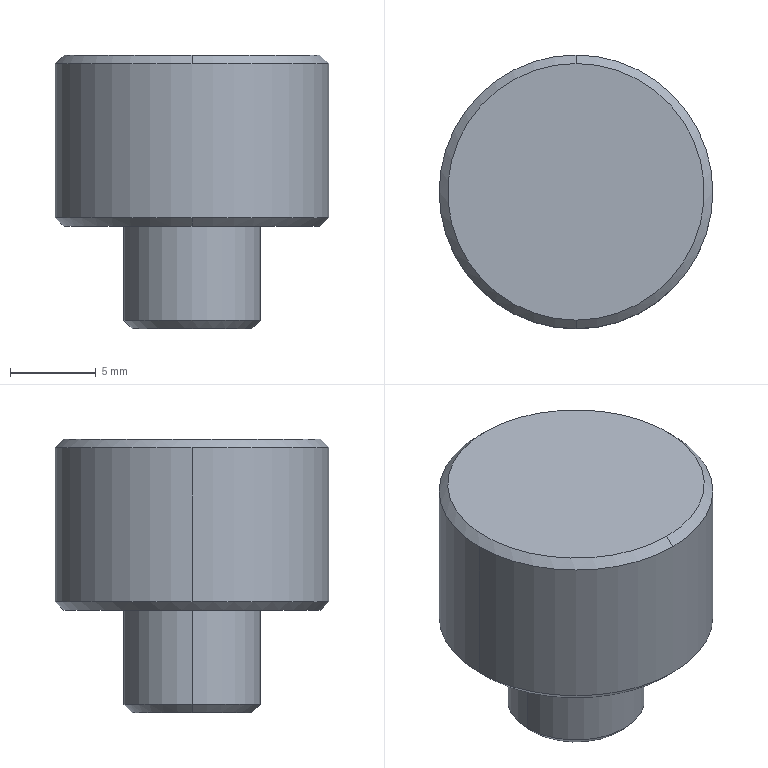Part | STEP file | fBY02F02M-00-12A | 1 solid | 13 faces | box 16 x 16 x 16 mm | volume 2297 mm3 | cone 6 | cylinder 4 | plane 3 | commonest cylinder face diameters 8 x2 16 x2
STEP:
#1=CARTESIAN_POINT('',(0.,0.,0.));
#2=DIRECTION('',(0.,0.,1.));
#3=DIRECTION('',(1.,0.,0.));
#4=AXIS2_PLACEMENT_3D('',#1,#2,#3);
#5=CARTESIAN_POINT('',(0.,8.,15.5));
#6=VERTEX_POINT('',#5);
#7=CARTESIAN_POINT('',(8.,0.,15.5));
#8=VERTEX_POINT('',#7);
#9=CARTESIAN_POINT('',(0.,0.,15.5));
#10=DIRECTION('',(0.,0.,-1.));
#11=DIRECTION('',(-1.,0.,0.));
#12=AXIS2_PLACEMENT_3D('',#9,#10,#11);
#13=CIRCLE('',#12,8.);
#14=CARTESIAN_POINT('',(0.,0.,16.));
#15=DIRECTION('',(0.,0.,-1.));
#16=DIRECTION('',(-1.,0.,0.));
#17=AXIS2_PLACEMENT_3D('',#14,#15,#16);
#18=CYLINDRICAL_SURFACE('',#17,8.);
#19=CARTESIAN_POINT('',(0.,0.5));
#20=DIRECTION('',(1.,0.));
#21=VECTOR('',#20,1.);
#22=LINE('',#19,#21);
#23=(GEOMETRIC_REPRESENTATION_CONTEXT(2)PARAMETRIC_REPRESENTATION_CONTEXT()REPRESENTATION_CONTEXT('',''));
#24=DEFINITIONAL_REPRESENTATION('',(#22),#23);
#25=PCURVE('',#18,#24);
#26=CARTESIAN_POINT('',(0.,0.,15.5));
#27=DIRECTION('',(0.,0.,-1.));
#28=DIRECTION('',(0.,1.,0.));
#29=AXIS2_PLACEMENT_3D('',#26,#27,#28);
#30=CONICAL_SURFACE('',#29,8.,0.7854);
#31=CARTESIAN_POINT('',(-1.571,0.));
#32=DIRECTION('',(1.,0.));
#33=VECTOR('',#32,1.);
#34=LINE('',#31,#33);
#35=(GEOMETRIC_REPRESENTATION_CONTEXT(2)PARAMETRIC_REPRESENTATION_CONTEXT()REPRESENTATION_CONTEXT('',''));
#36=DEFINITIONAL_REPRESENTATION('',(#34),#35);
#37=PCURVE('',#30,#36);
#38=SURFACE_CURVE('',#13,(#25,#37),.PCURVE_S1.);
#39=EDGE_CURVE('',#6,#8,#38,.T.);
#40=ORIENTED_EDGE('',*,*,#39,.T.);
#41=CARTESIAN_POINT('',(8.,0.,6.5));
#42=VERTEX_POINT('',#41);
#43=CARTESIAN_POINT('',(8.,0.,16.));
#44=DIRECTION('',(0.,0.,-1.));
#45=VECTOR('',#44,1.);
#46=LINE('',#43,#45);
#47=CARTESIAN_POINT('',(3.142,0.));
#48=DIRECTION('',(0.,1.));
#49=VECTOR('',#48,1.);
#50=LINE('',#47,#49);
#51=(GEOMETRIC_REPRESENTATION_CONTEXT(2)PARAMETRIC_REPRESENTATION_CONTEXT()REPRESENTATION_CONTEXT('',''));
#52=DEFINITIONAL_REPRESENTATION('',(#50),#51);
#53=PCURVE('',#18,#52);
#54=CARTESIAN_POINT('',(0.,0.,16.));
#55=DIRECTION('',(0.,0.,-1.));
#56=DIRECTION('',(-1.,0.,0.));
#57=AXIS2_PLACEMENT_3D('',#54,#55,#56);
#58=CYLINDRICAL_SURFACE('',#57,8.);
#59=CARTESIAN_POINT('',(3.142,0.));
#60=DIRECTION('',(0.,1.));
#61=VECTOR('',#60,1.);
#62=LINE('',#59,#61);
#63=(GEOMETRIC_REPRESENTATION_CONTEXT(2)PARAMETRIC_REPRESENTATION_CONTEXT()REPRESENTATION_CONTEXT('',''));
#64=DEFINITIONAL_REPRESENTATION('',(#62),#63);
#65=PCURVE('',#58,#64);
#66=SURFACE_CURVE('',#46,(#53,#65),.PCURVE_S1.);
#67=EDGE_CURVE('',#8,#42,#66,.T.);
#68=ORIENTED_EDGE('',*,*,#67,.T.);
#69=CARTESIAN_POINT('',(0.,8.,6.5));
#70=VERTEX_POINT('',#69);
#71=CARTESIAN_POINT('',(0.,0.,6.5));
#72=DIRECTION('',(0.,0.,1.));
#73=DIRECTION('',(-1.,0.,0.));
#74=AXIS2_PLACEMENT_3D('',#71,#72,#73);
#75=CIRCLE('',#74,8.);
#76=CARTESIAN_POINT('',(6.283,9.5));
#77=DIRECTION('',(-1.,0.));
#78=VECTOR('',#77,1.);
#79=LINE('',#76,#78);
#80=(GEOMETRIC_REPRESENTATION_CONTEXT(2)PARAMETRIC_REPRESENTATION_CONTEXT()REPRESENTATION_CONTEXT('',''));
#81=DEFINITIONAL_REPRESENTATION('',(#79),#80);
#82=PCURVE('',#18,#81);
#83=CARTESIAN_POINT('',(0.,0.,6.5));
#84=DIRECTION('',(0.,0.,1.));
#85=DIRECTION('',(0.,-1.,0.));
#86=AXIS2_PLACEMENT_3D('',#83,#84,#85);
#87=CONICAL_SURFACE('',#86,8.,0.7854);
#88=CARTESIAN_POINT('',(-1.571,0.));
#89=DIRECTION('',(1.,0.));
#90=VECTOR('',#89,1.);
#91=LINE('',#88,#90);
#92=(GEOMETRIC_REPRESENTATION_CONTEXT(2)PARAMETRIC_REPRESENTATION_CONTEXT()REPRESENTATION_CONTEXT('',''));
#93=DEFINITIONAL_REPRESENTATION('',(#91),#92);
#94=PCURVE('',#87,#93);
#95=SURFACE_CURVE('',#75,(#82,#94),.PCURVE_S1.);
#96=EDGE_CURVE('',#42,#70,#95,.T.);
#97=ORIENTED_EDGE('',*,*,#96,.T.);
#98=CARTESIAN_POINT('',(-8.,0.,6.5));
#99=VERTEX_POINT('',#98);
#100=CARTESIAN_POINT('',(0.,0.,6.5));
#101=DIRECTION('',(0.,0.,1.));
#102=DIRECTION('',(-1.,0.,0.));
#103=AXIS2_PLACEMENT_3D('',#100,#101,#102);
#104=CIRCLE('',#103,8.);
#105=CARTESIAN_POINT('',(6.283,9.5));
#106=DIRECTION('',(-1.,0.));
#107=VECTOR('',#106,1.);
#108=LINE('',#105,#107);
#109=(GEOMETRIC_REPRESENTATION_CONTEXT(2)PARAMETRIC_REPRESENTATION_CONTEXT()REPRESENTATION_CONTEXT('',''));
#110=DEFINITIONAL_REPRESENTATION('',(#108),#109);
#111=PCURVE('',#18,#110);
#112=CARTESIAN_POINT('',(0.,0.,6.5));
#113=DIRECTION('',(0.,0.,1.));
#114=DIRECTION('',(0.,-1.,0.));
#115=AXIS2_PLACEMENT_3D('',#112,#113,#114);
#116=CONICAL_SURFACE('',#115,8.,0.7854);
#117=CARTESIAN_POINT('',(-1.571,0.));
#118=DIRECTION('',(1.,0.));
#119=VECTOR('',#118,1.);
#120=LINE('',#117,#119);
#121=(GEOMETRIC_REPRESENTATION_CONTEXT(2)PARAMETRIC_REPRESENTATION_CONTEXT()REPRESENTATION_CONTEXT('',''));
#122=DEFINITIONAL_REPRESENTATION('',(#120),#121);
#123=PCURVE('',#116,#122);
#124=SURFACE_CURVE('',#104,(#111,#123),.PCURVE_S1.);
#125=EDGE_CURVE('',#70,#99,#124,.T.);
#126=ORIENTED_EDGE('',*,*,#125,.T.);
#127=CARTESIAN_POINT('',(-8.,0.,15.5));
#128=VERTEX_POINT('',#127);
#129=CARTESIAN_POINT('',(-8.,0.,16.));
#130=DIRECTION('',(0.,0.,-1.));
#131=VECTOR('',#130,1.);
#132=LINE('',#129,#131);
#133=CARTESIAN_POINT('',(0.,0.));
#134=DIRECTION('',(0.,1.));
#135=VECTOR('',#134,1.);
#136=LINE('',#133,#135);
#137=(GEOMETRIC_REPRESENTATION_CONTEXT(2)PARAMETRIC_REPRESENTATION_CONTEXT()REPRESENTATION_CONTEXT('',''));
#138=DEFINITIONAL_REPRESENTATION('',(#136),#137);
#139=PCURVE('',#18,#138);
#140=CARTESIAN_POINT('',(6.283,0.));
#141=DIRECTION('',(0.,1.));
#142=VECTOR('',#141,1.);
#143=LINE('',#140,#142);
#144=(GEOMETRIC_REPRESENTATION_CONTEXT(2)PARAMETRIC_REPRESENTATION_CONTEXT()REPRESENTATION_CONTEXT('',''));
#145=DEFINITIONAL_REPRESENTATION('',(#143),#144);
#146=PCURVE('',#58,#145);
#147=SURFACE_CURVE('',#132,(#139,#146),.PCURVE_S1.);
#148=EDGE_CURVE('',#128,#99,#147,.T.);
#149=ORIENTED_EDGE('',*,*,#148,.F.);
#150=CARTESIAN_POINT('',(0.,0.,15.5));
#151=DIRECTION('',(0.,0.,-1.));
#152=DIRECTION('',(-1.,0.,0.));
#153=AXIS2_PLACEMENT_3D('',#150,#151,#152);
#154=CIRCLE('',#153,8.);
#155=CARTESIAN_POINT('',(0.,0.5));
#156=DIRECTION('',(1.,0.));
#157=VECTOR('',#156,1.);
#158=LINE('',#155,#157);
#159=(GEOMETRIC_REPRESENTATION_CONTEXT(2)PARAMETRIC_REPRESENTATION_CONTEXT()REPRESENTATION_CONTEXT('',''));
#160=DEFINITIONAL_REPRESENTATION('',(#158),#159);
#161=PCURVE('',#18,#160);
#162=CARTESIAN_POINT('',(0.,0.,15.5));
#163=DIRECTION('',(0.,0.,-1.));
#164=DIRECTION('',(0.,1.,0.));
#165=AXIS2_PLACEMENT_3D('',#162,#163,#164);
#166=CONICAL_SURFACE('',#165,8.,0.7854);
#167=CARTESIAN_POINT('',(4.712,0.));
#168=DIRECTION('',(1.,0.));
#169=VECTOR('',#168,1.);
#170=LINE('',#167,#169);
#171=(GEOMETRIC_REPRESENTATION_CONTEXT(2)PARAMETRIC_REPRESENTATION_CONTEXT()REPRESENTATION_CONTEXT('',''));
#172=DEFINITIONAL_REPRESENTATION('',(#170),#171);
#173=PCURVE('',#166,#172);
#174=SURFACE_CURVE('',#154,(#161,#173),.PCURVE_S1.);
#175=EDGE_CURVE('',#128,#6,#174,.T.);
#176=ORIENTED_EDGE('',*,*,#175,.T.);
#177=EDGE_LOOP('',(#40,#68,#97,#126,#149,#176));
#178=FACE_BOUND('',#177,.T.);
#179=ADVANCED_FACE('',(#178),#18,.T.);
#180=CARTESIAN_POINT('',(0.,-7.5,6.));
#181=VERTEX_POINT('',#180);
#182=CARTESIAN_POINT('',(0.,7.5,6.));
#183=VERTEX_POINT('',#182);
#184=CARTESIAN_POINT('',(0.,0.,6.));
#185=DIRECTION('',(0.,0.,1.));
#186=DIRECTION('',(0.,-1.,0.));
#187=AXIS2_PLACEMENT_3D('',#184,#185,#186);
#188=CIRCLE('',#187,7.5);
#189=CARTESIAN_POINT('',(0.,-0.5));
#190=DIRECTION('',(1.,0.));
#191=VECTOR('',#190,1.);
#192=LINE('',#189,#191);
#193=(GEOMETRIC_REPRESENTATION_CONTEXT(2)PARAMETRIC_REPRESENTATION_CONTEXT()REPRESENTATION_CONTEXT('',''));
#194=DEFINITIONAL_REPRESENTATION('',(#192),#193);
#195=PCURVE('',#87,#194);
#196=CARTESIAN_POINT('',(0.,0.,6.));
#197=DIRECTION('',(0.,0.,1.));
#198=DIRECTION('',(1.,0.,0.));
#199=AXIS2_PLACEMENT_3D('',#196,#197,#198);
#200=PLANE('',#199);
#201=CARTESIAN_POINT('',(0.,0.));
#202=DIRECTION('',(0.,-1.));
#203=AXIS2_PLACEMENT_2D('',#201,#202);
#204=CIRCLE('',#203,7.5);
#205=(GEOMETRIC_REPRESENTATION_CONTEXT(2)PARAMETRIC_REPRESENTATION_CONTEXT()REPRESENTATION_CONTEXT('',''));
#206=DEFINITIONAL_REPRESENTATION('',(#204),#205);
#207=PCURVE('',#200,#206);
#208=SURFACE_CURVE('',#188,(#195,#207),.PCURVE_S1.);
#209=EDGE_CURVE('',#181,#183,#208,.T.);
#210=ORIENTED_EDGE('',*,*,#209,.T.);
#211=CARTESIAN_POINT('',(0.,8.,6.5));
#212=DIRECTION('',(0.,0.7071,0.7071));
#213=VECTOR('',#212,1.);
#214=LINE('',#211,#213);
#215=CARTESIAN_POINT('',(3.142,0.));
#216=DIRECTION('',(0.,1.));
#217=VECTOR('',#216,1.);
#218=LINE('',#215,#217);
#219=(GEOMETRIC_REPRESENTATION_CONTEXT(2)PARAMETRIC_REPRESENTATION_CONTEXT()REPRESENTATION_CONTEXT('',''));
#220=DEFINITIONAL_REPRESENTATION('',(#218),#219);
#221=PCURVE('',#87,#220);
#222=CARTESIAN_POINT('',(3.142,0.));
#223=DIRECTION('',(0.,1.));
#224=VECTOR('',#223,1.);
#225=LINE('',#222,#224);
#226=(GEOMETRIC_REPRESENTATION_CONTEXT(2)PARAMETRIC_REPRESENTATION_CONTEXT()REPRESENTATION_CONTEXT('',''));
#227=DEFINITIONAL_REPRESENTATION('',(#225),#226);
#228=PCURVE('',#116,#227);
#229=SURFACE_CURVE('',#214,(#221,#228),.PCURVE_S1.);
#230=EDGE_CURVE('',#183,#70,#229,.T.);
#231=ORIENTED_EDGE('',*,*,#230,.T.);
#232=ORIENTED_EDGE('',*,*,#96,.F.);
#233=CARTESIAN_POINT('',(0.,-8.,6.5));
#234=VERTEX_POINT('',#233);
#235=CARTESIAN_POINT('',(0.,0.,6.5));
#236=DIRECTION('',(0.,0.,1.));
#237=DIRECTION('',(-1.,0.,0.));
#238=AXIS2_PLACEMENT_3D('',#235,#236,#237);
#239=CIRCLE('',#238,8.);
#240=CARTESIAN_POINT('',(-1.571,0.));
#241=DIRECTION('',(1.,0.));
#242=VECTOR('',#241,1.);
#243=LINE('',#240,#242);
#244=(GEOMETRIC_REPRESENTATION_CONTEXT(2)PARAMETRIC_REPRESENTATION_CONTEXT()REPRESENTATION_CONTEXT('',''));
#245=DEFINITIONAL_REPRESENTATION('',(#243),#244);
#246=PCURVE('',#87,#245);
#247=CARTESIAN_POINT('',(6.283,9.5));
#248=DIRECTION('',(-1.,0.));
#249=VECTOR('',#248,1.);
#250=LINE('',#247,#249);
#251=(GEOMETRIC_REPRESENTATION_CONTEXT(2)PARAMETRIC_REPRESENTATION_CONTEXT()REPRESENTATION_CONTEXT('',''));
#252=DEFINITIONAL_REPRESENTATION('',(#250),#251);
#253=PCURVE('',#58,#252);
#254=SURFACE_CURVE('',#239,(#246,#253),.PCURVE_S1.);
#255=EDGE_CURVE('',#234,#42,#254,.T.);
#256=ORIENTED_EDGE('',*,*,#255,.F.);
#257=CARTESIAN_POINT('',(0.,-8.,6.5));
#258=DIRECTION('',(0.,-0.7071,0.7071));
#259=VECTOR('',#258,1.);
#260=LINE('',#257,#259);
#261=CARTESIAN_POINT('',(0.,0.));
#262=DIRECTION('',(0.,1.));
#263=VECTOR('',#262,1.);
#264=LINE('',#261,#263);
#265=(GEOMETRIC_REPRESENTATION_CONTEXT(2)PARAMETRIC_REPRESENTATION_CONTEXT()REPRESENTATION_CONTEXT('',''));
#266=DEFINITIONAL_REPRESENTATION('',(#264),#265);
#267=PCURVE('',#87,#266);
#268=CARTESIAN_POINT('',(6.283,0.));
#269=DIRECTION('',(0.,1.));
#270=VECTOR('',#269,1.);
#271=LINE('',#268,#270);
#272=(GEOMETRIC_REPRESENTATION_CONTEXT(2)PARAMETRIC_REPRESENTATION_CONTEXT()REPRESENTATION_CONTEXT('',''));
#273=DEFINITIONAL_REPRESENTATION('',(#271),#272);
#274=PCURVE('',#116,#273);
#275=SURFACE_CURVE('',#260,(#267,#274),.PCURVE_S1.);
#276=EDGE_CURVE('',#181,#234,#275,.T.);
#277=ORIENTED_EDGE('',*,*,#276,.F.);
#278=EDGE_LOOP('',(#210,#231,#232,#256,#277));
#279=FACE_BOUND('',#278,.T.);
#280=ADVANCED_FACE('',(#279),#87,.T.);
#281=CARTESIAN_POINT('',(0.,7.5,16.));
#282=VERTEX_POINT('',#281);
#283=CARTESIAN_POINT('',(0.,-7.5,16.));
#284=VERTEX_POINT('',#283);
#285=CARTESIAN_POINT('',(0.,0.,16.));
#286=DIRECTION('',(0.,0.,-1.));
#287=DIRECTION('',(0.,1.,0.));
#288=AXIS2_PLACEMENT_3D('',#285,#286,#287);
#289=CIRCLE('',#288,7.5);
#290=CARTESIAN_POINT('',(0.,-0.5));
#291=DIRECTION('',(1.,0.));
#292=VECTOR('',#291,1.);
#293=LINE('',#290,#292);
#294=(GEOMETRIC_REPRESENTATION_CONTEXT(2)PARAMETRIC_REPRESENTATION_CONTEXT()REPRESENTATION_CONTEXT('',''));
#295=DEFINITIONAL_REPRESENTATION('',(#293),#294);
#296=PCURVE('',#30,#295);
#297=CARTESIAN_POINT('',(0.,0.,16.));
#298=DIRECTION('',(0.,0.,1.));
#299=DIRECTION('',(1.,0.,0.));
#300=AXIS2_PLACEMENT_3D('',#297,#298,#299);
#301=PLANE('',#300);
#302=CARTESIAN_POINT('',(0.,7.5));
#303=CARTESIAN_POINT('',(12.99,7.5));
#304=CARTESIAN_POINT('',(6.495,-3.75));
#305=CARTESIAN_POINT('',(0.,-15.));
#306=CARTESIAN_POINT('',(-6.495,-3.75));
#307=CARTESIAN_POINT('',(-12.99,7.5));
#308=CARTESIAN_POINT('',(0.,7.5));
#309=(BOUNDED_CURVE()B_SPLINE_CURVE(2,(#302,#303,#304,#305,#306,#307,#308),.UNSPECIFIED.,.T.,.F.)B_SPLINE_CURVE_WITH_KNOTS((1,2,2,2,2,1),(-2.094,0.,2.094,4.189,6.283,8.378),.UNSPECIFIED.)CURVE()GEOMETRIC_REPRESENTATION_ITEM()RATIONAL_B_SPLINE_CURVE((1.,0.5,1.,0.5,1.,0.5,1.))REPRESENTATION_ITEM(''));
#310=(GEOMETRIC_REPRESENTATION_CONTEXT(2)PARAMETRIC_REPRESENTATION_CONTEXT()REPRESENTATION_CONTEXT('',''));
#311=DEFINITIONAL_REPRESENTATION('',(#309),#310);
#312=PCURVE('',#301,#311);
#313=SURFACE_CURVE('',#289,(#296,#312),.PCURVE_S1.);
#314=EDGE_CURVE('',#282,#284,#313,.T.);
#315=ORIENTED_EDGE('',*,*,#314,.T.);
#316=CARTESIAN_POINT('',(0.,-8.,15.5));
#317=VERTEX_POINT('',#316);
#318=CARTESIAN_POINT('',(0.,-8.,15.5));
#319=DIRECTION('',(0.,-0.7071,-0.7071));
#320=VECTOR('',#319,1.);
#321=LINE('',#318,#320);
#322=CARTESIAN_POINT('',(3.142,0.));
#323=DIRECTION('',(0.,1.));
#324=VECTOR('',#323,1.);
#325=LINE('',#322,#324);
#326=(GEOMETRIC_REPRESENTATION_CONTEXT(2)PARAMETRIC_REPRESENTATION_CONTEXT()REPRESENTATION_CONTEXT('',''));
#327=DEFINITIONAL_REPRESENTATION('',(#325),#326);
#328=PCURVE('',#30,#327);
#329=CARTESIAN_POINT('',(3.142,0.));
#330=DIRECTION('',(0.,1.));
#331=VECTOR('',#330,1.);
#332=LINE('',#329,#331);
#333=(GEOMETRIC_REPRESENTATION_CONTEXT(2)PARAMETRIC_REPRESENTATION_CONTEXT()REPRESENTATION_CONTEXT('',''));
#334=DEFINITIONAL_REPRESENTATION('',(#332),#333);
#335=PCURVE('',#166,#334);
#336=SURFACE_CURVE('',#321,(#328,#335),.PCURVE_S1.);
#337=EDGE_CURVE('',#284,#317,#336,.T.);
#338=ORIENTED_EDGE('',*,*,#337,.T.);
#339=CARTESIAN_POINT('',(0.,0.,15.5));
#340=DIRECTION('',(0.,0.,-1.));
#341=DIRECTION('',(-1.,0.,0.));
#342=AXIS2_PLACEMENT_3D('',#339,#340,#341);
#343=CIRCLE('',#342,8.);
#344=CARTESIAN_POINT('',(-1.571,0.));
#345=DIRECTION('',(1.,0.));
#346=VECTOR('',#345,1.);
#347=LINE('',#344,#346);
#348=(GEOMETRIC_REPRESENTATION_CONTEXT(2)PARAMETRIC_REPRESENTATION_CONTEXT()REPRESENTATION_CONTEXT('',''));
#349=DEFINITIONAL_REPRESENTATION('',(#347),#348);
#350=PCURVE('',#30,#349);
#351=CARTESIAN_POINT('',(0.,0.5));
#352=DIRECTION('',(1.,0.));
#353=VECTOR('',#352,1.);
#354=LINE('',#351,#353);
#355=(GEOMETRIC_REPRESENTATION_CONTEXT(2)PARAMETRIC_REPRESENTATION_CONTEXT()REPRESENTATION_CONTEXT('',''));
#356=DEFINITIONAL_REPRESENTATION('',(#354),#355);
#357=PCURVE('',#58,#356);
#358=SURFACE_CURVE('',#343,(#350,#357),.PCURVE_S1.);
#359=EDGE_CURVE('',#8,#317,#358,.T.);
#360=ORIENTED_EDGE('',*,*,#359,.F.);
#361=ORIENTED_EDGE('',*,*,#39,.F.);
#362=CARTESIAN_POINT('',(0.,8.,15.5));
#363=DIRECTION('',(0.,0.7071,-0.7071));
#364=VECTOR('',#363,1.);
#365=LINE('',#362,#364);
#366=CARTESIAN_POINT('',(0.,0.));
#367=DIRECTION('',(0.,1.));
#368=VECTOR('',#367,1.);
#369=LINE('',#366,#368);
#370=(GEOMETRIC_REPRESENTATION_CONTEXT(2)PARAMETRIC_REPRESENTATION_CONTEXT()REPRESENTATION_CONTEXT('',''));
#371=DEFINITIONAL_REPRESENTATION('',(#369),#370);
#372=PCURVE('',#30,#371);
#373=CARTESIAN_POINT('',(6.283,0.));
#374=DIRECTION('',(0.,1.));
#375=VECTOR('',#374,1.);
#376=LINE('',#373,#375);
#377=(GEOMETRIC_REPRESENTATION_CONTEXT(2)PARAMETRIC_REPRESENTATION_CONTEXT()REPRESENTATION_CONTEXT('',''));
#378=DEFINITIONAL_REPRESENTATION('',(#376),#377);
#379=PCURVE('',#166,#378);
#380=SURFACE_CURVE('',#365,(#372,#379),.PCURVE_S1.);
#381=EDGE_CURVE('',#282,#6,#380,.T.);
#382=ORIENTED_EDGE('',*,*,#381,.F.);
#383=EDGE_LOOP('',(#315,#338,#360,#361,#382));
#384=FACE_BOUND('',#383,.T.);
#385=ADVANCED_FACE('',(#384),#30,.T.);
#386=CARTESIAN_POINT('',(-4.,0.,6.));
#387=VERTEX_POINT('',#386);
#388=CARTESIAN_POINT('',(4.,0.,6.));
#389=VERTEX_POINT('',#388);
#390=CARTESIAN_POINT('',(0.,0.,6.));
#391=DIRECTION('',(0.,0.,-1.));
#392=DIRECTION('',(-1.,0.,0.));
#393=AXIS2_PLACEMENT_3D('',#390,#391,#392);
#394=CIRCLE('',#393,4.);
#395=CARTESIAN_POINT('',(0.,0.,6.));
#396=DIRECTION('',(0.,0.,-1.));
#397=DIRECTION('',(-1.,0.,0.));
#398=AXIS2_PLACEMENT_3D('',#395,#396,#397);
#399=CYLINDRICAL_SURFACE('',#398,4.);
#400=CARTESIAN_POINT('',(0.,0.));
#401=DIRECTION('',(1.,0.));
#402=VECTOR('',#401,1.);
#403=LINE('',#400,#402);
#404=(GEOMETRIC_REPRESENTATION_CONTEXT(2)PARAMETRIC_REPRESENTATION_CONTEXT()REPRESENTATION_CONTEXT('',''));
#405=DEFINITIONAL_REPRESENTATION('',(#403),#404);
#406=PCURVE('',#399,#405);
#407=CARTESIAN_POINT('',(-4.,0.));
#408=CARTESIAN_POINT('',(-4.,6.928));
#409=CARTESIAN_POINT('',(2.,3.464));
#410=CARTESIAN_POINT('',(8.,0.));
#411=CARTESIAN_POINT('',(2.,-3.464));
#412=CARTESIAN_POINT('',(-4.,-6.928));
#413=CARTESIAN_POINT('',(-4.,0.));
#414=(BOUNDED_CURVE()B_SPLINE_CURVE(2,(#407,#408,#409,#410,#411,#412,#413),.UNSPECIFIED.,.T.,.F.)B_SPLINE_CURVE_WITH_KNOTS((1,2,2,2,2,1),(-2.094,0.,2.094,4.189,6.283,8.378),.UNSPECIFIED.)CURVE()GEOMETRIC_REPRESENTATION_ITEM()RATIONAL_B_SPLINE_CURVE((1.,0.5,1.,0.5,1.,0.5,1.))REPRESENTATION_ITEM(''));
#415=(GEOMETRIC_REPRESENTATION_CONTEXT(2)PARAMETRIC_REPRESENTATION_CONTEXT()REPRESENTATION_CONTEXT('',''));
#416=DEFINITIONAL_REPRESENTATION('',(#414),#415);
#417=PCURVE('',#200,#416);
#418=SURFACE_CURVE('',#394,(#406,#417),.PCURVE_S1.);
#419=EDGE_CURVE('',#387,#389,#418,.T.);
#420=ORIENTED_EDGE('',*,*,#419,.T.);
#421=CARTESIAN_POINT('',(4.,0.,0.5));
#422=VERTEX_POINT('',#421);
#423=CARTESIAN_POINT('',(4.,0.,6.));
#424=DIRECTION('',(0.,0.,-1.));
#425=VECTOR('',#424,1.);
#426=LINE('',#423,#425);
#427=CARTESIAN_POINT('',(3.142,0.));
#428=DIRECTION('',(0.,1.));
#429=VECTOR('',#428,1.);
#430=LINE('',#427,#429);
#431=(GEOMETRIC_REPRESENTATION_CONTEXT(2)PARAMETRIC_REPRESENTATION_CONTEXT()REPRESENTATION_CONTEXT('',''));
#432=DEFINITIONAL_REPRESENTATION('',(#430),#431);
#433=PCURVE('',#399,#432);
#434=CARTESIAN_POINT('',(0.,0.,6.));
#435=DIRECTION('',(0.,0.,-1.));
#436=DIRECTION('',(-1.,0.,0.));
#437=AXIS2_PLACEMENT_3D('',#434,#435,#436);
#438=CYLINDRICAL_SURFACE('',#437,4.);
#439=CARTESIAN_POINT('',(3.142,0.));
#440=DIRECTION('',(0.,1.));
#441=VECTOR('',#440,1.);
#442=LINE('',#439,#441);
#443=(GEOMETRIC_REPRESENTATION_CONTEXT(2)PARAMETRIC_REPRESENTATION_CONTEXT()REPRESENTATION_CONTEXT('',''));
#444=DEFINITIONAL_REPRESENTATION('',(#442),#443);
#445=PCURVE('',#438,#444);
#446=SURFACE_CURVE('',#426,(#433,#445),.PCURVE_S1.);
#447=EDGE_CURVE('',#389,#422,#446,.T.);
#448=ORIENTED_EDGE('',*,*,#447,.T.);
#449=CARTESIAN_POINT('',(-4.,0.,0.5));
#450=VERTEX_POINT('',#449);
#451=CARTESIAN_POINT('',(0.,0.,0.5));
#452=DIRECTION('',(0.,0.,1.));
#453=DIRECTION('',(-1.,0.,0.));
#454=AXIS2_PLACEMENT_3D('',#451,#452,#453);
#455=CIRCLE('',#454,4.);
#456=CARTESIAN_POINT('',(6.283,5.5));
#457=DIRECTION('',(-1.,0.));
#458=VECTOR('',#457,1.);
#459=LINE('',#456,#458);
#460=(GEOMETRIC_REPRESENTATION_CONTEXT(2)PARAMETRIC_REPRESENTATION_CONTEXT()REPRESENTATION_CONTEXT('',''));
#461=DEFINITIONAL_REPRESENTATION('',(#459),#460);
#462=PCURVE('',#399,#461);
#463=CARTESIAN_POINT('',(0.,0.,0.5));
#464=DIRECTION('',(0.,0.,1.));
#465=DIRECTION('',(1.,0.,0.));
#466=AXIS2_PLACEMENT_3D('',#463,#464,#465);
#467=CONICAL_SURFACE('',#466,4.,0.7854);
#468=CARTESIAN_POINT('',(-3.142,0.));
#469=DIRECTION('',(1.,0.));
#470=VECTOR('',#469,1.);
#471=LINE('',#468,#470);
#472=(GEOMETRIC_REPRESENTATION_CONTEXT(2)PARAMETRIC_REPRESENTATION_CONTEXT()REPRESENTATION_CONTEXT('',''));
#473=DEFINITIONAL_REPRESENTATION('',(#471),#472);
#474=PCURVE('',#467,#473);
#475=SURFACE_CURVE('',#455,(#462,#474),.PCURVE_S1.);
#476=EDGE_CURVE('',#422,#450,#475,.T.);
#477=ORIENTED_EDGE('',*,*,#476,.T.);
#478=CARTESIAN_POINT('',(-4.,0.,6.));
#479=DIRECTION('',(0.,0.,-1.));
#480=VECTOR('',#479,1.);
#481=LINE('',#478,#480);
#482=CARTESIAN_POINT('',(0.,0.));
#483=DIRECTION('',(0.,1.));
#484=VECTOR('',#483,1.);
#485=LINE('',#482,#484);
#486=(GEOMETRIC_REPRESENTATION_CONTEXT(2)PARAMETRIC_REPRESENTATION_CONTEXT()REPRESENTATION_CONTEXT('',''));
#487=DEFINITIONAL_REPRESENTATION('',(#485),#486);
#488=PCURVE('',#399,#487);
#489=CARTESIAN_POINT('',(6.283,0.));
#490=DIRECTION('',(0.,1.));
#491=VECTOR('',#490,1.);
#492=LINE('',#489,#491);
#493=(GEOMETRIC_REPRESENTATION_CONTEXT(2)PARAMETRIC_REPRESENTATION_CONTEXT()REPRESENTATION_CONTEXT('',''));
#494=DEFINITIONAL_REPRESENTATION('',(#492),#493);
#495=PCURVE('',#438,#494);
#496=SURFACE_CURVE('',#481,(#488,#495),.PCURVE_S1.);
#497=EDGE_CURVE('',#387,#450,#496,.T.);
#498=ORIENTED_EDGE('',*,*,#497,.F.);
#499=EDGE_LOOP('',(#420,#448,#477,#498));
#500=FACE_BOUND('',#499,.T.);
#501=ADVANCED_FACE('',(#500),#399,.T.);
#502=CARTESIAN_POINT('',(3.5,0.,0.));
#503=VERTEX_POINT('',#502);
#504=CARTESIAN_POINT('',(-3.5,0.,0.));
#505=VERTEX_POINT('',#504);
#506=CARTESIAN_POINT('',(0.,0.,0.));
#507=DIRECTION('',(0.,0.,1.));
#508=DIRECTION('',(1.,0.,0.));
#509=AXIS2_PLACEMENT_3D('',#506,#507,#508);
#510=CIRCLE('',#509,3.5);
#511=CARTESIAN_POINT('',(0.,-0.5));
#512=DIRECTION('',(1.,0.));
#513=VECTOR('',#512,1.);
#514=LINE('',#511,#513);
#515=(GEOMETRIC_REPRESENTATION_CONTEXT(2)PARAMETRIC_REPRESENTATION_CONTEXT()REPRESENTATION_CONTEXT('',''));
#516=DEFINITIONAL_REPRESENTATION('',(#514),#515);
#517=PCURVE('',#467,#516);
#518=CARTESIAN_POINT('',(0.,0.,0.));
#519=DIRECTION('',(0.,0.,1.));
#520=DIRECTION('',(1.,0.,0.));
#521=AXIS2_PLACEMENT_3D('',#518,#519,#520);
#522=PLANE('',#521);
#523=CARTESIAN_POINT('',(0.,0.));
#524=DIRECTION('',(1.,0.));
#525=AXIS2_PLACEMENT_2D('',#523,#524);
#526=CIRCLE('',#525,3.5);
#527=(GEOMETRIC_REPRESENTATION_CONTEXT(2)PARAMETRIC_REPRESENTATION_CONTEXT()REPRESENTATION_CONTEXT('',''));
#528=DEFINITIONAL_REPRESENTATION('',(#526),#527);
#529=PCURVE('',#522,#528);
#530=SURFACE_CURVE('',#510,(#517,#529),.PCURVE_S1.);
#531=EDGE_CURVE('',#503,#505,#530,.T.);
#532=ORIENTED_EDGE('',*,*,#531,.T.);
#533=CARTESIAN_POINT('',(-4.,0.,0.5));
#534=DIRECTION('',(-0.7071,0.,0.7071));
#535=VECTOR('',#534,1.);
#536=LINE('',#533,#535);
#537=CARTESIAN_POINT('',(3.142,0.));
#538=DIRECTION('',(0.,1.));
#539=VECTOR('',#538,1.);
#540=LINE('',#537,#539);
#541=(GEOMETRIC_REPRESENTATION_CONTEXT(2)PARAMETRIC_REPRESENTATION_CONTEXT()REPRESENTATION_CONTEXT('',''));
#542=DEFINITIONAL_REPRESENTATION('',(#540),#541);
#543=PCURVE('',#467,#542);
#544=CARTESIAN_POINT('',(0.,0.,0.5));
#545=DIRECTION('',(0.,0.,1.));
#546=DIRECTION('',(1.,0.,0.));
#547=AXIS2_PLACEMENT_3D('',#544,#545,#546);
#548=CONICAL_SURFACE('',#547,4.,0.7854);
#549=CARTESIAN_POINT('',(3.142,0.));
#550=DIRECTION('',(0.,1.));
#551=VECTOR('',#550,1.);
#552=LINE('',#549,#551);
#553=(GEOMETRIC_REPRESENTATION_CONTEXT(2)PARAMETRIC_REPRESENTATION_CONTEXT()REPRESENTATION_CONTEXT('',''));
#554=DEFINITIONAL_REPRESENTATION('',(#552),#553);
#555=PCURVE('',#548,#554);
#556=SURFACE_CURVE('',#536,(#543,#555),.PCURVE_S1.);
#557=EDGE_CURVE('',#505,#450,#556,.T.);
#558=ORIENTED_EDGE('',*,*,#557,.T.);
#559=ORIENTED_EDGE('',*,*,#476,.F.);
#560=CARTESIAN_POINT('',(4.,0.,0.5));
#561=DIRECTION('',(0.7071,0.,0.7071));
#562=VECTOR('',#561,1.);
#563=LINE('',#560,#562);
#564=CARTESIAN_POINT('',(0.,0.));
#565=DIRECTION('',(0.,1.));
#566=VECTOR('',#565,1.);
#567=LINE('',#564,#566);
#568=(GEOMETRIC_REPRESENTATION_CONTEXT(2)PARAMETRIC_REPRESENTATION_CONTEXT()REPRESENTATION_CONTEXT('',''));
#569=DEFINITIONAL_REPRESENTATION('',(#567),#568);
#570=PCURVE('',#467,#569);
#571=CARTESIAN_POINT('',(6.283,0.));
#572=DIRECTION('',(0.,1.));
#573=VECTOR('',#572,1.);
#574=LINE('',#571,#573);
#575=(GEOMETRIC_REPRESENTATION_CONTEXT(2)PARAMETRIC_REPRESENTATION_CONTEXT()REPRESENTATION_CONTEXT('',''));
#576=DEFINITIONAL_REPRESENTATION('',(#574),#575);
#577=PCURVE('',#548,#576);
#578=SURFACE_CURVE('',#563,(#570,#577),.PCURVE_S1.);
#579=EDGE_CURVE('',#503,#422,#578,.T.);
#580=ORIENTED_EDGE('',*,*,#579,.F.);
#581=EDGE_LOOP('',(#532,#558,#559,#580));
#582=FACE_BOUND('',#581,.T.);
#583=ADVANCED_FACE('',(#582),#467,.T.);
#584=ORIENTED_EDGE('',*,*,#67,.F.);
#585=ORIENTED_EDGE('',*,*,#359,.T.);
#586=CARTESIAN_POINT('',(0.,0.,15.5));
#587=DIRECTION('',(0.,0.,-1.));
#588=DIRECTION('',(-1.,0.,0.));
#589=AXIS2_PLACEMENT_3D('',#586,#587,#588);
#590=CIRCLE('',#589,8.);
#591=CARTESIAN_POINT('',(0.,0.5));
#592=DIRECTION('',(1.,0.));
#593=VECTOR('',#592,1.);
#594=LINE('',#591,#593);
#595=(GEOMETRIC_REPRESENTATION_CONTEXT(2)PARAMETRIC_REPRESENTATION_CONTEXT()REPRESENTATION_CONTEXT('',''));
#596=DEFINITIONAL_REPRESENTATION('',(#594),#595);
#597=PCURVE('',#58,#596);
#598=CARTESIAN_POINT('',(-1.571,0.));
#599=DIRECTION('',(1.,0.));
#600=VECTOR('',#599,1.);
#601=LINE('',#598,#600);
#602=(GEOMETRIC_REPRESENTATION_CONTEXT(2)PARAMETRIC_REPRESENTATION_CONTEXT()REPRESENTATION_CONTEXT('',''));
#603=DEFINITIONAL_REPRESENTATION('',(#601),#602);
#604=PCURVE('',#166,#603);
#605=SURFACE_CURVE('',#590,(#597,#604),.PCURVE_S1.);
#606=EDGE_CURVE('',#317,#128,#605,.T.);
#607=ORIENTED_EDGE('',*,*,#606,.T.);
#608=ORIENTED_EDGE('',*,*,#148,.T.);
#609=CARTESIAN_POINT('',(0.,0.,6.5));
#610=DIRECTION('',(0.,0.,1.));
#611=DIRECTION('',(-1.,0.,0.));
#612=AXIS2_PLACEMENT_3D('',#609,#610,#611);
#613=CIRCLE('',#612,8.);
#614=CARTESIAN_POINT('',(6.283,9.5));
#615=DIRECTION('',(-1.,0.));
#616=VECTOR('',#615,1.);
#617=LINE('',#614,#616);
#618=(GEOMETRIC_REPRESENTATION_CONTEXT(2)PARAMETRIC_REPRESENTATION_CONTEXT()REPRESENTATION_CONTEXT('',''));
#619=DEFINITIONAL_REPRESENTATION('',(#617),#618);
#620=PCURVE('',#58,#619);
#621=CARTESIAN_POINT('',(4.712,0.));
#622=DIRECTION('',(1.,0.));
#623=VECTOR('',#622,1.);
#624=LINE('',#621,#623);
#625=(GEOMETRIC_REPRESENTATION_CONTEXT(2)PARAMETRIC_REPRESENTATION_CONTEXT()REPRESENTATION_CONTEXT('',''));
#626=DEFINITIONAL_REPRESENTATION('',(#624),#625);
#627=PCURVE('',#116,#626);
#628=SURFACE_CURVE('',#613,(#620,#627),.PCURVE_S1.);
#629=EDGE_CURVE('',#99,#234,#628,.T.);
#630=ORIENTED_EDGE('',*,*,#629,.T.);
#631=ORIENTED_EDGE('',*,*,#255,.T.);
#632=EDGE_LOOP('',(#584,#585,#607,#608,#630,#631));
#633=FACE_BOUND('',#632,.T.);
#634=ADVANCED_FACE('',(#633),#58,.T.);
#635=ORIENTED_EDGE('',*,*,#230,.F.);
#636=CARTESIAN_POINT('',(0.,0.,6.));
#637=DIRECTION('',(0.,0.,1.));
#638=DIRECTION('',(0.,-1.,0.));
#639=AXIS2_PLACEMENT_3D('',#636,#637,#638);
#640=CIRCLE('',#639,7.5);
#641=CARTESIAN_POINT('',(0.,-0.5));
#642=DIRECTION('',(1.,0.));
#643=VECTOR('',#642,1.);
#644=LINE('',#641,#643);
#645=(GEOMETRIC_REPRESENTATION_CONTEXT(2)PARAMETRIC_REPRESENTATION_CONTEXT()REPRESENTATION_CONTEXT('',''));
#646=DEFINITIONAL_REPRESENTATION('',(#644),#645);
#647=PCURVE('',#116,#646);
#648=CARTESIAN_POINT('',(0.,0.));
#649=DIRECTION('',(0.,-1.));
#650=AXIS2_PLACEMENT_2D('',#648,#649);
#651=CIRCLE('',#650,7.5);
#652=(GEOMETRIC_REPRESENTATION_CONTEXT(2)PARAMETRIC_REPRESENTATION_CONTEXT()REPRESENTATION_CONTEXT('',''));
#653=DEFINITIONAL_REPRESENTATION('',(#651),#652);
#654=PCURVE('',#200,#653);
#655=SURFACE_CURVE('',#640,(#647,#654),.PCURVE_S1.);
#656=EDGE_CURVE('',#183,#181,#655,.T.);
#657=ORIENTED_EDGE('',*,*,#656,.T.);
#658=ORIENTED_EDGE('',*,*,#276,.T.);
#659=ORIENTED_EDGE('',*,*,#629,.F.);
#660=ORIENTED_EDGE('',*,*,#125,.F.);
#661=EDGE_LOOP('',(#635,#657,#658,#659,#660));
#662=FACE_BOUND('',#661,.T.);
#663=ADVANCED_FACE('',(#662),#116,.T.);
#664=ORIENTED_EDGE('',*,*,#337,.F.);
#665=CARTESIAN_POINT('',(0.,0.,16.));
#666=DIRECTION('',(0.,0.,-1.));
#667=DIRECTION('',(0.,1.,0.));
#668=AXIS2_PLACEMENT_3D('',#665,#666,#667);
#669=CIRCLE('',#668,7.5);
#670=CARTESIAN_POINT('',(0.,-0.5));
#671=DIRECTION('',(1.,0.));
#672=VECTOR('',#671,1.);
#673=LINE('',#670,#672);
#674=(GEOMETRIC_REPRESENTATION_CONTEXT(2)PARAMETRIC_REPRESENTATION_CONTEXT()REPRESENTATION_CONTEXT('',''));
#675=DEFINITIONAL_REPRESENTATION('',(#673),#674);
#676=PCURVE('',#166,#675);
#677=CARTESIAN_POINT('',(0.,7.5));
#678=CARTESIAN_POINT('',(12.99,7.5));
#679=CARTESIAN_POINT('',(6.495,-3.75));
#680=CARTESIAN_POINT('',(0.,-15.));
#681=CARTESIAN_POINT('',(-6.495,-3.75));
#682=CARTESIAN_POINT('',(-12.99,7.5));
#683=CARTESIAN_POINT('',(0.,7.5));
#684=(BOUNDED_CURVE()B_SPLINE_CURVE(2,(#677,#678,#679,#680,#681,#682,#683),.UNSPECIFIED.,.T.,.F.)B_SPLINE_CURVE_WITH_KNOTS((1,2,2,2,2,1),(-2.094,0.,2.094,4.189,6.283,8.378),.UNSPECIFIED.)CURVE()GEOMETRIC_REPRESENTATION_ITEM()RATIONAL_B_SPLINE_CURVE((1.,0.5,1.,0.5,1.,0.5,1.))REPRESENTATION_ITEM(''));
#685=(GEOMETRIC_REPRESENTATION_CONTEXT(2)PARAMETRIC_REPRESENTATION_CONTEXT()REPRESENTATION_CONTEXT('',''));
#686=DEFINITIONAL_REPRESENTATION('',(#684),#685);
#687=PCURVE('',#301,#686);
#688=SURFACE_CURVE('',#669,(#676,#687),.PCURVE_S1.);
#689=EDGE_CURVE('',#284,#282,#688,.T.);
#690=ORIENTED_EDGE('',*,*,#689,.T.);
#691=ORIENTED_EDGE('',*,*,#381,.T.);
#692=ORIENTED_EDGE('',*,*,#175,.F.);
#693=ORIENTED_EDGE('',*,*,#606,.F.);
#694=EDGE_LOOP('',(#664,#690,#691,#692,#693));
#695=FACE_BOUND('',#694,.T.);
#696=ADVANCED_FACE('',(#695),#166,.T.);
#697=ORIENTED_EDGE('',*,*,#419,.F.);
#698=CARTESIAN_POINT('',(0.,0.,6.));
#699=DIRECTION('',(0.,0.,-1.));
#700=DIRECTION('',(-1.,0.,0.));
#701=AXIS2_PLACEMENT_3D('',#698,#699,#700);
#702=CIRCLE('',#701,4.);
#703=CARTESIAN_POINT('',(-4.,0.));
#704=CARTESIAN_POINT('',(-4.,6.928));
#705=CARTESIAN_POINT('',(2.,3.464));
#706=CARTESIAN_POINT('',(8.,0.));
#707=CARTESIAN_POINT('',(2.,-3.464));
#708=CARTESIAN_POINT('',(-4.,-6.928));
#709=CARTESIAN_POINT('',(-4.,0.));
#710=(BOUNDED_CURVE()B_SPLINE_CURVE(2,(#703,#704,#705,#706,#707,#708,#709),.UNSPECIFIED.,.T.,.F.)B_SPLINE_CURVE_WITH_KNOTS((1,2,2,2,2,1),(-2.094,0.,2.094,4.189,6.283,8.378),.UNSPECIFIED.)CURVE()GEOMETRIC_REPRESENTATION_ITEM()RATIONAL_B_SPLINE_CURVE((1.,0.5,1.,0.5,1.,0.5,1.))REPRESENTATION_ITEM(''));
#711=(GEOMETRIC_REPRESENTATION_CONTEXT(2)PARAMETRIC_REPRESENTATION_CONTEXT()REPRESENTATION_CONTEXT('',''));
#712=DEFINITIONAL_REPRESENTATION('',(#710),#711);
#713=PCURVE('',#200,#712);
#714=CARTESIAN_POINT('',(0.,0.));
#715=DIRECTION('',(1.,0.));
#716=VECTOR('',#715,1.);
#717=LINE('',#714,#716);
#718=(GEOMETRIC_REPRESENTATION_CONTEXT(2)PARAMETRIC_REPRESENTATION_CONTEXT()REPRESENTATION_CONTEXT('',''));
#719=DEFINITIONAL_REPRESENTATION('',(#717),#718);
#720=PCURVE('',#438,#719);
#721=SURFACE_CURVE('',#702,(#713,#720),.PCURVE_S1.);
#722=EDGE_CURVE('',#389,#387,#721,.T.);
#723=ORIENTED_EDGE('',*,*,#722,.F.);
#724=EDGE_LOOP('',(#697,#723));
#725=FACE_BOUND('',#724,.T.);
#726=ORIENTED_EDGE('',*,*,#209,.F.);
#727=ORIENTED_EDGE('',*,*,#656,.F.);
#728=EDGE_LOOP('',(#726,#727));
#729=FACE_BOUND('',#728,.T.);
#730=ADVANCED_FACE('',(#725,#729),#200,.F.);
#731=ORIENTED_EDGE('',*,*,#314,.F.);
#732=ORIENTED_EDGE('',*,*,#689,.F.);
#733=EDGE_LOOP('',(#731,#732));
#734=FACE_BOUND('',#733,.T.);
#735=ADVANCED_FACE('',(#734),#301,.T.);
#736=ORIENTED_EDGE('',*,*,#447,.F.);
#737=ORIENTED_EDGE('',*,*,#722,.T.);
#738=ORIENTED_EDGE('',*,*,#497,.T.);
#739=CARTESIAN_POINT('',(0.,0.,0.5));
#740=DIRECTION('',(0.,0.,1.));
#741=DIRECTION('',(-1.,0.,0.));
#742=AXIS2_PLACEMENT_3D('',#739,#740,#741);
#743=CIRCLE('',#742,4.);
#744=CARTESIAN_POINT('',(6.283,5.5));
#745=DIRECTION('',(-1.,0.));
#746=VECTOR('',#745,1.);
#747=LINE('',#744,#746);
#748=(GEOMETRIC_REPRESENTATION_CONTEXT(2)PARAMETRIC_REPRESENTATION_CONTEXT()REPRESENTATION_CONTEXT('',''));
#749=DEFINITIONAL_REPRESENTATION('',(#747),#748);
#750=PCURVE('',#438,#749);
#751=CARTESIAN_POINT('',(3.142,0.));
#752=DIRECTION('',(1.,0.));
#753=VECTOR('',#752,1.);
#754=LINE('',#751,#753);
#755=(GEOMETRIC_REPRESENTATION_CONTEXT(2)PARAMETRIC_REPRESENTATION_CONTEXT()REPRESENTATION_CONTEXT('',''));
#756=DEFINITIONAL_REPRESENTATION('',(#754),#755);
#757=PCURVE('',#548,#756);
#758=SURFACE_CURVE('',#743,(#750,#757),.PCURVE_S1.);
#759=EDGE_CURVE('',#450,#422,#758,.T.);
#760=ORIENTED_EDGE('',*,*,#759,.T.);
#761=EDGE_LOOP('',(#736,#737,#738,#760));
#762=FACE_BOUND('',#761,.T.);
#763=ADVANCED_FACE('',(#762),#438,.T.);
#764=ORIENTED_EDGE('',*,*,#557,.F.);
#765=CARTESIAN_POINT('',(0.,0.,0.));
#766=DIRECTION('',(0.,0.,1.));
#767=DIRECTION('',(1.,0.,0.));
#768=AXIS2_PLACEMENT_3D('',#765,#766,#767);
#769=CIRCLE('',#768,3.5);
#770=CARTESIAN_POINT('',(0.,-0.5));
#771=DIRECTION('',(1.,0.));
#772=VECTOR('',#771,1.);
#773=LINE('',#770,#772);
#774=(GEOMETRIC_REPRESENTATION_CONTEXT(2)PARAMETRIC_REPRESENTATION_CONTEXT()REPRESENTATION_CONTEXT('',''));
#775=DEFINITIONAL_REPRESENTATION('',(#773),#774);
#776=PCURVE('',#548,#775);
#777=CARTESIAN_POINT('',(0.,0.));
#778=DIRECTION('',(1.,0.));
#779=AXIS2_PLACEMENT_2D('',#777,#778);
#780=CIRCLE('',#779,3.5);
#781=(GEOMETRIC_REPRESENTATION_CONTEXT(2)PARAMETRIC_REPRESENTATION_CONTEXT()REPRESENTATION_CONTEXT('',''));
#782=DEFINITIONAL_REPRESENTATION('',(#780),#781);
#783=PCURVE('',#522,#782);
#784=SURFACE_CURVE('',#769,(#776,#783),.PCURVE_S1.);
#785=EDGE_CURVE('',#505,#503,#784,.T.);
#786=ORIENTED_EDGE('',*,*,#785,.T.);
#787=ORIENTED_EDGE('',*,*,#579,.T.);
#788=ORIENTED_EDGE('',*,*,#759,.F.);
#789=EDGE_LOOP('',(#764,#786,#787,#788));
#790=FACE_BOUND('',#789,.T.);
#791=ADVANCED_FACE('',(#790),#548,.T.);
#792=ORIENTED_EDGE('',*,*,#531,.F.);
#793=ORIENTED_EDGE('',*,*,#785,.F.);
#794=EDGE_LOOP('',(#792,#793));
#795=FACE_BOUND('',#794,.T.);
#796=ADVANCED_FACE('',(#795),#522,.F.);
#797=CLOSED_SHELL('',(#179,#280,#385,#501,#583,#634,#663,#696,#730,#735,#763,#791,#796));
#798=MANIFOLD_SOLID_BREP('',#797);
#799=(LENGTH_UNIT()NAMED_UNIT(*)SI_UNIT(.MILLI.,.METRE.));
#800=UNCERTAINTY_MEASURE_WITH_UNIT(LENGTH_MEASURE(0.0000001),#799,'','');
#801=(NAMED_UNIT(*)PLANE_ANGLE_UNIT()SI_UNIT($,.RADIAN.));
#802=(NAMED_UNIT(*)SI_UNIT($,.STERADIAN.)SOLID_ANGLE_UNIT());
#803=(GEOMETRIC_REPRESENTATION_CONTEXT(3)GLOBAL_UNCERTAINTY_ASSIGNED_CONTEXT((#800))GLOBAL_UNIT_ASSIGNED_CONTEXT((#799,#801,#802))REPRESENTATION_CONTEXT('',''));
#804=ADVANCED_BREP_SHAPE_REPRESENTATION('',(#4,#798),#803);